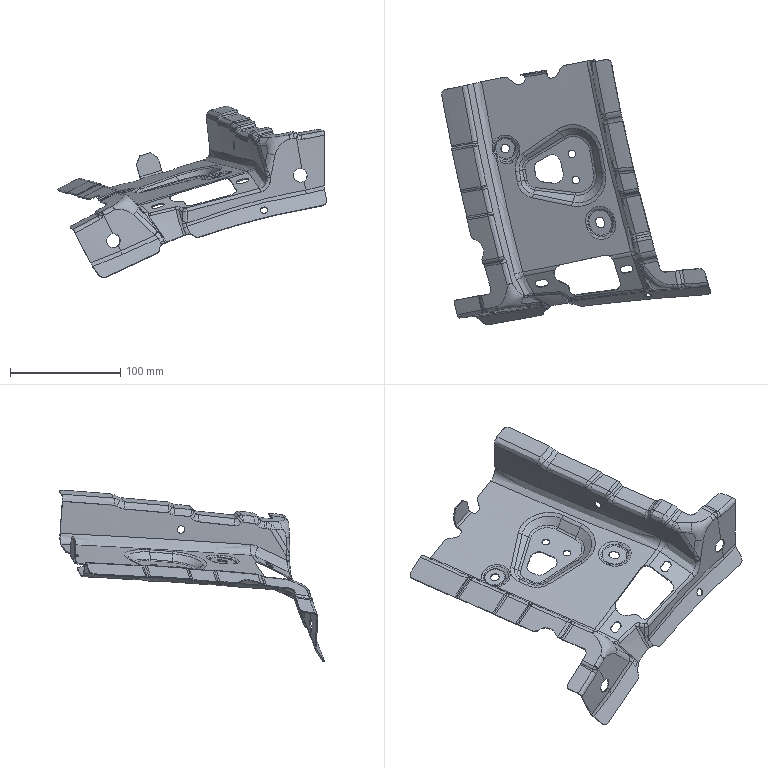Part | STEP file | FNA5401411 | 1 solid | 567 faces | box 243.972 x 240.219 x 155.739 mm | volume 51999 mm3 | spline 492 | plane 29 | cylinder 26 | other 12 | sphere 8 | commonest cylinder face diameters 7 x12 8 x4 4 x2 6 x2 14 x2 16 x2